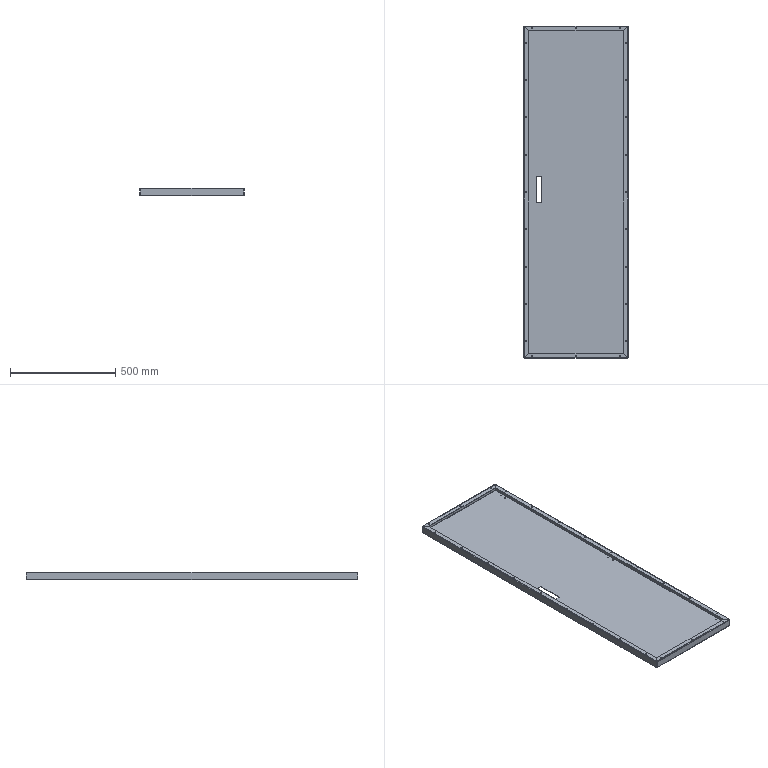Part | SolidWorks | 1 solid | 134 faces | box 494.5 x 1578 x 37 mm | volume 2481313 mm3 | cylinder 76 | plane 42 | spline 16 | commonest cylinder face diameters 5 x60 1.473 x8 6.473 x8